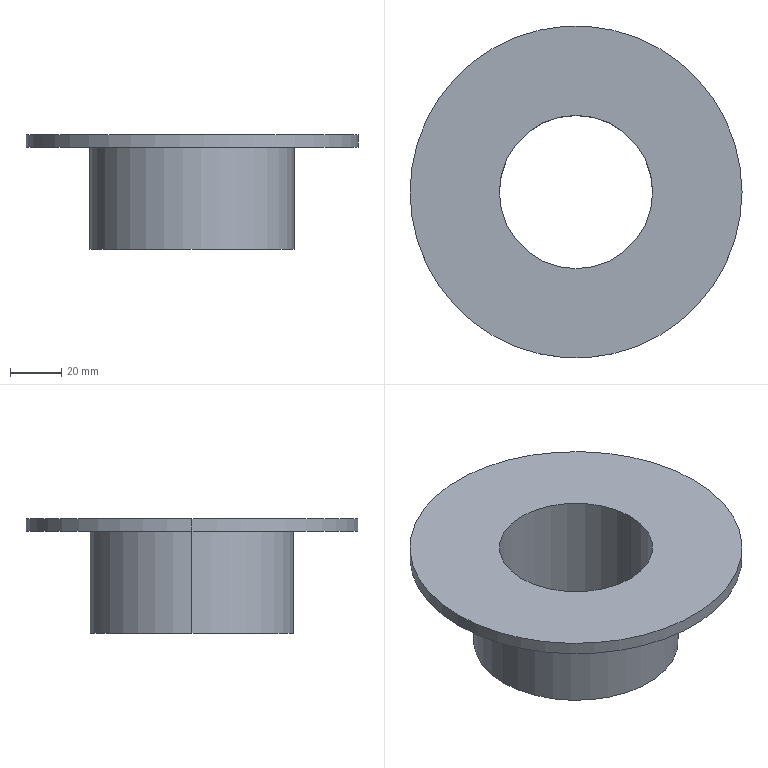Part | SolidWorks | features Extrusion 1, ICE 1 | 1 solid | 9 faces | box 130 x 130 x 45 mm | volume 140194 mm3 | cylinder 6 | plane 3 | commonest cylinder face diameters 60 x2 80 x2 130 x2
STEP:
#1=CARTESIAN_POINT('',(65.,0.,45.));
#2=VERTEX_POINT('',#1);
#3=CARTESIAN_POINT('',(-65.,0.,45.));
#4=VERTEX_POINT('',#3);
#5=CARTESIAN_POINT('',(0.,0.,45.));
#6=DIRECTION('',(0.,0.,1.));
#7=DIRECTION('',(1.,0.,0.));
#8=AXIS2_PLACEMENT_3D('',#5,#6,#7);
#9=CIRCLE('',#8,65.);
#10=EDGE_CURVE('',#2,#4,#9,.T.);
#11=ORIENTED_EDGE('',*,*,#10,.F.);
#12=CARTESIAN_POINT('',(65.,0.,40.));
#13=VERTEX_POINT('',#12);
#14=CARTESIAN_POINT('',(65.,0.,45.));
#15=DIRECTION('',(0.,0.,-1.));
#16=VECTOR('',#15,1000.);
#17=LINE('',#14,#16);
#18=EDGE_CURVE('',#2,#13,#17,.T.);
#19=ORIENTED_EDGE('',*,*,#18,.T.);
#20=CARTESIAN_POINT('',(-65.,0.,40.));
#21=VERTEX_POINT('',#20);
#22=CARTESIAN_POINT('',(0.,0.,40.));
#23=DIRECTION('',(0.,0.,1.));
#24=DIRECTION('',(1.,0.,0.));
#25=AXIS2_PLACEMENT_3D('',#22,#23,#24);
#26=CIRCLE('',#25,65.);
#27=EDGE_CURVE('',#13,#21,#26,.T.);
#28=ORIENTED_EDGE('',*,*,#27,.T.);
#29=CARTESIAN_POINT('',(-65.,0.,45.));
#30=DIRECTION('',(0.,0.,-1.));
#31=VECTOR('',#30,1000.);
#32=LINE('',#29,#31);
#33=EDGE_CURVE('',#4,#21,#32,.T.);
#34=ORIENTED_EDGE('',*,*,#33,.F.);
#35=EDGE_LOOP('',(#11,#19,#28,#34));
#36=FACE_OUTER_BOUND('',#35,.T.);
#37=CARTESIAN_POINT('',(0.,0.,45.));
#38=DIRECTION('',(0.,0.,-1.));
#39=DIRECTION('',(-1.,0.,0.));
#40=AXIS2_PLACEMENT_3D('',#37,#38,#39);
#41=CYLINDRICAL_SURFACE('',#40,65.);
#42=ADVANCED_FACE('',(#36),#41,.T.);
#43=CARTESIAN_POINT('',(-30.,0.,45.));
#44=VERTEX_POINT('',#43);
#45=CARTESIAN_POINT('',(30.,0.,45.));
#46=VERTEX_POINT('',#45);
#47=CARTESIAN_POINT('',(0.,0.,45.));
#48=DIRECTION('',(0.,0.,1.));
#49=DIRECTION('',(1.,0.,0.));
#50=AXIS2_PLACEMENT_3D('',#47,#48,#49);
#51=CIRCLE('',#50,30.);
#52=EDGE_CURVE('',#44,#46,#51,.T.);
#53=ORIENTED_EDGE('',*,*,#52,.T.);
#54=CARTESIAN_POINT('',(30.,0.,0.));
#55=VERTEX_POINT('',#54);
#56=CARTESIAN_POINT('',(30.,0.,40.));
#57=DIRECTION('',(0.,0.,-1.));
#58=VECTOR('',#57,1000.);
#59=LINE('',#56,#58);
#60=EDGE_CURVE('',#46,#55,#59,.T.);
#61=ORIENTED_EDGE('',*,*,#60,.T.);
#62=CARTESIAN_POINT('',(-30.,0.,0.));
#63=VERTEX_POINT('',#62);
#64=CARTESIAN_POINT('',(0.,0.,0.));
#65=DIRECTION('',(0.,0.,1.));
#66=DIRECTION('',(1.,0.,0.));
#67=AXIS2_PLACEMENT_3D('',#64,#65,#66);
#68=CIRCLE('',#67,30.);
#69=EDGE_CURVE('',#63,#55,#68,.T.);
#70=ORIENTED_EDGE('',*,*,#69,.F.);
#71=CARTESIAN_POINT('',(-30.,0.,40.));
#72=DIRECTION('',(0.,0.,-1.));
#73=VECTOR('',#72,1000.);
#74=LINE('',#71,#73);
#75=EDGE_CURVE('',#44,#63,#74,.T.);
#76=ORIENTED_EDGE('',*,*,#75,.F.);
#77=EDGE_LOOP('',(#53,#61,#70,#76));
#78=FACE_OUTER_BOUND('',#77,.T.);
#79=CARTESIAN_POINT('',(0.,0.,40.));
#80=DIRECTION('',(0.,0.,-1.));
#81=DIRECTION('',(-1.,0.,0.));
#82=AXIS2_PLACEMENT_3D('',#79,#80,#81);
#83=CYLINDRICAL_SURFACE('',#82,30.);
#84=ADVANCED_FACE('',(#78),#83,.F.);
#85=CARTESIAN_POINT('',(40.,0.,40.));
#86=VERTEX_POINT('',#85);
#87=CARTESIAN_POINT('',(-40.,0.,40.));
#88=VERTEX_POINT('',#87);
#89=CARTESIAN_POINT('',(0.,0.,40.));
#90=DIRECTION('',(0.,0.,1.));
#91=DIRECTION('',(1.,0.,0.));
#92=AXIS2_PLACEMENT_3D('',#89,#90,#91);
#93=CIRCLE('',#92,40.);
#94=EDGE_CURVE('',#86,#88,#93,.T.);
#95=ORIENTED_EDGE('',*,*,#94,.F.);
#96=CARTESIAN_POINT('',(40.,0.,0.));
#97=VERTEX_POINT('',#96);
#98=CARTESIAN_POINT('',(40.,0.,40.));
#99=DIRECTION('',(0.,0.,-1.));
#100=VECTOR('',#99,1000.);
#101=LINE('',#98,#100);
#102=EDGE_CURVE('',#86,#97,#101,.T.);
#103=ORIENTED_EDGE('',*,*,#102,.T.);
#104=CARTESIAN_POINT('',(-40.,0.,0.));
#105=VERTEX_POINT('',#104);
#106=CARTESIAN_POINT('',(0.,0.,0.));
#107=DIRECTION('',(0.,0.,1.));
#108=DIRECTION('',(1.,0.,0.));
#109=AXIS2_PLACEMENT_3D('',#106,#107,#108);
#110=CIRCLE('',#109,40.);
#111=EDGE_CURVE('',#97,#105,#110,.T.);
#112=ORIENTED_EDGE('',*,*,#111,.T.);
#113=CARTESIAN_POINT('',(-40.,0.,40.));
#114=DIRECTION('',(0.,0.,-1.));
#115=VECTOR('',#114,1000.);
#116=LINE('',#113,#115);
#117=EDGE_CURVE('',#88,#105,#116,.T.);
#118=ORIENTED_EDGE('',*,*,#117,.F.);
#119=EDGE_LOOP('',(#95,#103,#112,#118));
#120=FACE_OUTER_BOUND('',#119,.T.);
#121=CARTESIAN_POINT('',(0.,0.,40.));
#122=DIRECTION('',(0.,0.,-1.));
#123=DIRECTION('',(-1.,0.,0.));
#124=AXIS2_PLACEMENT_3D('',#121,#122,#123);
#125=CYLINDRICAL_SURFACE('',#124,40.);
#126=ADVANCED_FACE('',(#120),#125,.T.);
#127=CARTESIAN_POINT('',(0.,0.,0.));
#128=DIRECTION('',(0.,0.,1.));
#129=DIRECTION('',(1.,0.,0.));
#130=AXIS2_PLACEMENT_3D('',#127,#128,#129);
#131=CIRCLE('',#130,40.);
#132=EDGE_CURVE('',#105,#97,#131,.T.);
#133=ORIENTED_EDGE('',*,*,#132,.F.);
#134=ORIENTED_EDGE('',*,*,#111,.F.);
#135=EDGE_LOOP('',(#133,#134));
#136=FACE_OUTER_BOUND('',#135,.T.);
#137=ORIENTED_EDGE('',*,*,#69,.T.);
#138=CARTESIAN_POINT('',(0.,0.,0.));
#139=DIRECTION('',(0.,0.,1.));
#140=DIRECTION('',(1.,0.,0.));
#141=AXIS2_PLACEMENT_3D('',#138,#139,#140);
#142=CIRCLE('',#141,30.);
#143=EDGE_CURVE('',#55,#63,#142,.T.);
#144=ORIENTED_EDGE('',*,*,#143,.T.);
#145=EDGE_LOOP('',(#137,#144));
#146=FACE_BOUND('',#145,.T.);
#147=CARTESIAN_POINT('',(0.,0.,0.));
#148=DIRECTION('',(0.,0.,1.));
#149=DIRECTION('',(1.,0.,0.));
#150=AXIS2_PLACEMENT_3D('',#147,#148,#149);
#151=PLANE('',#150);
#152=ADVANCED_FACE('',(#136,#146),#151,.F.);
#153=ORIENTED_EDGE('',*,*,#102,.F.);
#154=CARTESIAN_POINT('',(0.,0.,40.));
#155=DIRECTION('',(0.,0.,1.));
#156=DIRECTION('',(1.,0.,0.));
#157=AXIS2_PLACEMENT_3D('',#154,#155,#156);
#158=CIRCLE('',#157,40.);
#159=EDGE_CURVE('',#88,#86,#158,.T.);
#160=ORIENTED_EDGE('',*,*,#159,.F.);
#161=ORIENTED_EDGE('',*,*,#117,.T.);
#162=ORIENTED_EDGE('',*,*,#132,.T.);
#163=EDGE_LOOP('',(#153,#160,#161,#162));
#164=FACE_OUTER_BOUND('',#163,.T.);
#165=CARTESIAN_POINT('',(0.,0.,40.));
#166=DIRECTION('',(0.,0.,-1.));
#167=DIRECTION('',(-1.,0.,0.));
#168=AXIS2_PLACEMENT_3D('',#165,#166,#167);
#169=CYLINDRICAL_SURFACE('',#168,40.);
#170=ADVANCED_FACE('',(#164),#169,.T.);
#171=ORIENTED_EDGE('',*,*,#60,.F.);
#172=CARTESIAN_POINT('',(0.,0.,45.));
#173=DIRECTION('',(0.,0.,1.));
#174=DIRECTION('',(1.,0.,0.));
#175=AXIS2_PLACEMENT_3D('',#172,#173,#174);
#176=CIRCLE('',#175,30.);
#177=EDGE_CURVE('',#46,#44,#176,.T.);
#178=ORIENTED_EDGE('',*,*,#177,.T.);
#179=ORIENTED_EDGE('',*,*,#75,.T.);
#180=ORIENTED_EDGE('',*,*,#143,.F.);
#181=EDGE_LOOP('',(#171,#178,#179,#180));
#182=FACE_OUTER_BOUND('',#181,.T.);
#183=CARTESIAN_POINT('',(0.,0.,40.));
#184=DIRECTION('',(0.,0.,-1.));
#185=DIRECTION('',(-1.,0.,0.));
#186=AXIS2_PLACEMENT_3D('',#183,#184,#185);
#187=CYLINDRICAL_SURFACE('',#186,30.);
#188=ADVANCED_FACE('',(#182),#187,.F.);
#189=CARTESIAN_POINT('',(0.,0.,40.));
#190=DIRECTION('',(0.,0.,1.));
#191=DIRECTION('',(1.,0.,0.));
#192=AXIS2_PLACEMENT_3D('',#189,#190,#191);
#193=CIRCLE('',#192,65.);
#194=EDGE_CURVE('',#21,#13,#193,.T.);
#195=ORIENTED_EDGE('',*,*,#194,.F.);
#196=ORIENTED_EDGE('',*,*,#27,.F.);
#197=EDGE_LOOP('',(#195,#196));
#198=FACE_OUTER_BOUND('',#197,.T.);
#199=ORIENTED_EDGE('',*,*,#159,.T.);
#200=ORIENTED_EDGE('',*,*,#94,.T.);
#201=EDGE_LOOP('',(#199,#200));
#202=FACE_BOUND('',#201,.T.);
#203=CARTESIAN_POINT('',(0.,0.,40.));
#204=DIRECTION('',(0.,0.,1.));
#205=DIRECTION('',(1.,0.,0.));
#206=AXIS2_PLACEMENT_3D('',#203,#204,#205);
#207=PLANE('',#206);
#208=ADVANCED_FACE('',(#198,#202),#207,.F.);
#209=CARTESIAN_POINT('',(0.,0.,45.));
#210=DIRECTION('',(0.,0.,1.));
#211=DIRECTION('',(1.,0.,0.));
#212=AXIS2_PLACEMENT_3D('',#209,#210,#211);
#213=CIRCLE('',#212,65.);
#214=EDGE_CURVE('',#4,#2,#213,.T.);
#215=ORIENTED_EDGE('',*,*,#214,.T.);
#216=ORIENTED_EDGE('',*,*,#10,.T.);
#217=EDGE_LOOP('',(#215,#216));
#218=FACE_OUTER_BOUND('',#217,.T.);
#219=ORIENTED_EDGE('',*,*,#52,.F.);
#220=ORIENTED_EDGE('',*,*,#177,.F.);
#221=EDGE_LOOP('',(#219,#220));
#222=FACE_BOUND('',#221,.T.);
#223=CARTESIAN_POINT('',(0.,0.,45.));
#224=DIRECTION('',(0.,0.,1.));
#225=DIRECTION('',(1.,0.,0.));
#226=AXIS2_PLACEMENT_3D('',#223,#224,#225);
#227=PLANE('',#226);
#228=ADVANCED_FACE('',(#218,#222),#227,.T.);
#229=ORIENTED_EDGE('',*,*,#18,.F.);
#230=ORIENTED_EDGE('',*,*,#214,.F.);
#231=ORIENTED_EDGE('',*,*,#33,.T.);
#232=ORIENTED_EDGE('',*,*,#194,.T.);
#233=EDGE_LOOP('',(#229,#230,#231,#232));
#234=FACE_OUTER_BOUND('',#233,.T.);
#235=CARTESIAN_POINT('',(0.,0.,45.));
#236=DIRECTION('',(0.,0.,-1.));
#237=DIRECTION('',(-1.,0.,0.));
#238=AXIS2_PLACEMENT_3D('',#235,#236,#237);
#239=CYLINDRICAL_SURFACE('',#238,65.);
#240=ADVANCED_FACE('',(#234),#239,.T.);
#241=CLOSED_SHELL('',(#42,#84,#126,#152,#170,#188,#208,#228,#240));
#242=MANIFOLD_SOLID_BREP('',#241);
#243=CARTESIAN_POINT('',(0.,0.,0.));
#244=DIRECTION('',(0.,0.,1.));
#245=DIRECTION('',(1.,0.,0.));
#246=AXIS2_PLACEMENT_3D('',#243,#244,#245);
#247=(LENGTH_UNIT()NAMED_UNIT(*)SI_UNIT(.MILLI.,.METRE.));
#248=UNCERTAINTY_MEASURE_WITH_UNIT(LENGTH_MEASURE(0.00001),#247,'','');
#249=(NAMED_UNIT(*)PLANE_ANGLE_UNIT()SI_UNIT($,.RADIAN.));
#250=(NAMED_UNIT(*)SI_UNIT($,.STERADIAN.)SOLID_ANGLE_UNIT());
#251=(GEOMETRIC_REPRESENTATION_CONTEXT(3)GLOBAL_UNCERTAINTY_ASSIGNED_CONTEXT((#248))GLOBAL_UNIT_ASSIGNED_CONTEXT((#247,#249,#250))REPRESENTATION_CONTEXT('',''));
#252=ADVANCED_BREP_SHAPE_REPRESENTATION('',(#242,#246),#251);